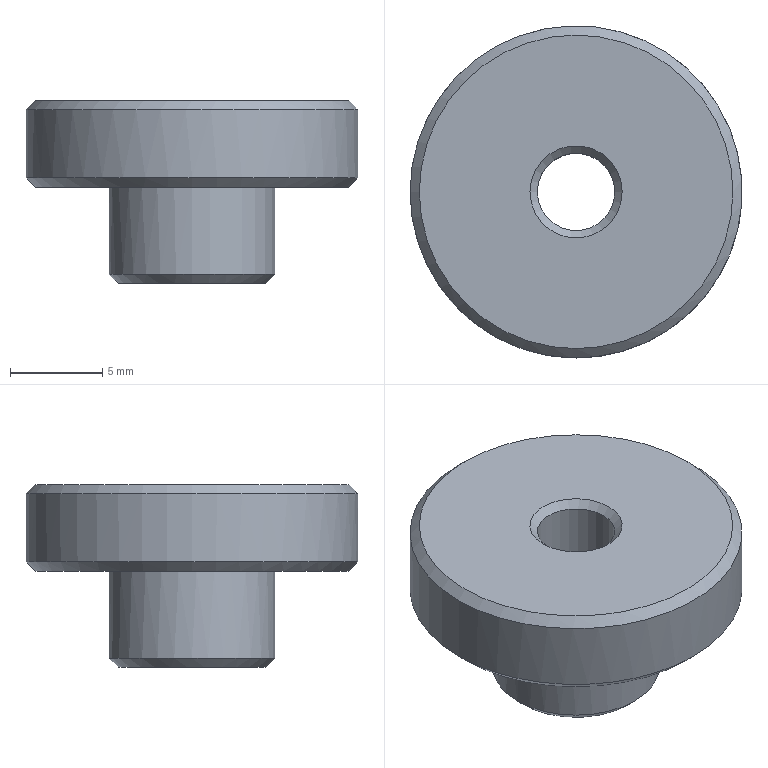Part | STEP file | 1 solid | 11 faces | box 18 x 18 x 9.92 mm | volume 1371 mm3 | cone 5 | cylinder 3 | plane 3 | commonest cylinder face diameters 4.2 x1 9 x1 18 x1
STEP:
#1=CARTESIAN_POINT('',(0.,0.,0.));
#2=DIRECTION('',(0.,0.,1.));
#3=DIRECTION('',(1.,0.,0.));
#4=AXIS2_PLACEMENT_3D('',#1,#2,#3);
#5=CARTESIAN_POINT('',(1716.457,442.48,-42.801));
#6=VERTEX_POINT('',#5);
#7=CARTESIAN_POINT('',(1720.957,437.98,-42.801));
#8=VERTEX_POINT('',#7);
#9=CARTESIAN_POINT('',(1720.957,442.48,-42.801));
#10=DIRECTION('',(0.,0.,1.));
#11=DIRECTION('',(-1.,0.,0.));
#12=AXIS2_PLACEMENT_3D('',#9,#10,#11);
#13=CIRCLE('',#12,4.5);
#14=CARTESIAN_POINT('',(1720.957,442.48,-44.081));
#15=DIRECTION('',(0.,0.,1.));
#16=DIRECTION('',(1.,0.,0.));
#17=AXIS2_PLACEMENT_3D('',#14,#15,#16);
#18=CYLINDRICAL_SURFACE('',#17,4.5);
#19=CARTESIAN_POINT('',(9.425,1.28));
#20=DIRECTION('',(1.,0.));
#21=VECTOR('',#20,1.);
#22=LINE('',#19,#21);
#23=(GEOMETRIC_REPRESENTATION_CONTEXT(2)PARAMETRIC_REPRESENTATION_CONTEXT()REPRESENTATION_CONTEXT('',''));
#24=DEFINITIONAL_REPRESENTATION('',(#22),#23);
#25=PCURVE('',#18,#24);
#26=CARTESIAN_POINT('',(1720.957,442.48,-43.301));
#27=DIRECTION('',(0.,0.,1.));
#28=DIRECTION('',(1.,0.,0.));
#29=AXIS2_PLACEMENT_3D('',#26,#27,#28);
#30=CONICAL_SURFACE('',#29,4.,0.7854);
#31=CARTESIAN_POINT('',(9.425,0.5));
#32=DIRECTION('',(1.,0.));
#33=VECTOR('',#32,1.);
#34=LINE('',#31,#33);
#35=(GEOMETRIC_REPRESENTATION_CONTEXT(2)PARAMETRIC_REPRESENTATION_CONTEXT()REPRESENTATION_CONTEXT('',''));
#36=DEFINITIONAL_REPRESENTATION('',(#34),#35);
#37=PCURVE('',#30,#36);
#38=SURFACE_CURVE('',#13,(#25,#37),.PCURVE_S1.);
#39=EDGE_CURVE('',#6,#8,#38,.T.);
#40=ORIENTED_EDGE('',*,*,#39,.T.);
#41=CARTESIAN_POINT('',(1720.957,437.98,-38.081));
#42=VERTEX_POINT('',#41);
#43=CARTESIAN_POINT('',(1720.957,437.98,-42.801));
#44=CARTESIAN_POINT('',(1720.957,437.98,-38.081));
#45=B_SPLINE_CURVE_WITH_KNOTS('',1,(#43,#44),.UNSPECIFIED.,.F.,.F.,(2,2),(1.28,6.),.PIECEWISE_BEZIER_KNOTS.);
#46=CARTESIAN_POINT('',(10.996,0.));
#47=DIRECTION('',(0.,1.));
#48=VECTOR('',#47,1.);
#49=LINE('',#46,#48);
#50=(GEOMETRIC_REPRESENTATION_CONTEXT(2)PARAMETRIC_REPRESENTATION_CONTEXT()REPRESENTATION_CONTEXT('',''));
#51=DEFINITIONAL_REPRESENTATION('',(#49),#50);
#52=PCURVE('',#18,#51);
#53=CARTESIAN_POINT('',(4.712,0.));
#54=DIRECTION('',(0.,1.));
#55=VECTOR('',#54,1.);
#56=LINE('',#53,#55);
#57=(GEOMETRIC_REPRESENTATION_CONTEXT(2)PARAMETRIC_REPRESENTATION_CONTEXT()REPRESENTATION_CONTEXT('',''));
#58=DEFINITIONAL_REPRESENTATION('',(#56),#57);
#59=PCURVE('',#18,#58);
#60=SEAM_CURVE('',#45,(#52,#59),.PCURVE_S1.);
#61=EDGE_CURVE('',#8,#42,#60,.T.);
#62=ORIENTED_EDGE('',*,*,#61,.T.);
#63=CARTESIAN_POINT('',(1720.957,442.48,-38.081));
#64=DIRECTION('',(0.,0.,-1.));
#65=DIRECTION('',(0.,-1.,0.));
#66=AXIS2_PLACEMENT_3D('',#63,#64,#65);
#67=CIRCLE('',#66,4.5);
#68=CARTESIAN_POINT('',(10.996,6.));
#69=DIRECTION('',(-1.,0.));
#70=VECTOR('',#69,1.);
#71=LINE('',#68,#70);
#72=(GEOMETRIC_REPRESENTATION_CONTEXT(2)PARAMETRIC_REPRESENTATION_CONTEXT()REPRESENTATION_CONTEXT('',''));
#73=DEFINITIONAL_REPRESENTATION('',(#71),#72);
#74=PCURVE('',#18,#73);
#75=CARTESIAN_POINT('',(1720.957,442.48,-38.081));
#76=DIRECTION('',(0.,0.,-1.));
#77=DIRECTION('',(0.,-1.,0.));
#78=AXIS2_PLACEMENT_3D('',#75,#76,#77);
#79=PLANE('',#78);
#80=CARTESIAN_POINT('',(0.,0.));
#81=DIRECTION('',(1.,0.));
#82=AXIS2_PLACEMENT_2D('',#80,#81);
#83=CIRCLE('',#82,4.5);
#84=(GEOMETRIC_REPRESENTATION_CONTEXT(2)PARAMETRIC_REPRESENTATION_CONTEXT()REPRESENTATION_CONTEXT('',''));
#85=DEFINITIONAL_REPRESENTATION('',(#83),#84);
#86=PCURVE('',#79,#85);
#87=SURFACE_CURVE('',#67,(#74,#86),.PCURVE_S1.);
#88=EDGE_CURVE('',#42,#42,#87,.T.);
#89=ORIENTED_EDGE('',*,*,#88,.T.);
#90=ORIENTED_EDGE('',*,*,#61,.F.);
#91=CARTESIAN_POINT('',(1720.957,442.48,-42.801));
#92=DIRECTION('',(0.,0.,1.));
#93=DIRECTION('',(-1.,0.,0.));
#94=AXIS2_PLACEMENT_3D('',#91,#92,#93);
#95=CIRCLE('',#94,4.5);
#96=CARTESIAN_POINT('',(3.142,1.28));
#97=DIRECTION('',(1.,0.));
#98=VECTOR('',#97,1.);
#99=LINE('',#96,#98);
#100=(GEOMETRIC_REPRESENTATION_CONTEXT(2)PARAMETRIC_REPRESENTATION_CONTEXT()REPRESENTATION_CONTEXT('',''));
#101=DEFINITIONAL_REPRESENTATION('',(#99),#100);
#102=PCURVE('',#18,#101);
#103=CARTESIAN_POINT('',(3.142,0.5));
#104=DIRECTION('',(1.,0.));
#105=VECTOR('',#104,1.);
#106=LINE('',#103,#105);
#107=(GEOMETRIC_REPRESENTATION_CONTEXT(2)PARAMETRIC_REPRESENTATION_CONTEXT()REPRESENTATION_CONTEXT('',''));
#108=DEFINITIONAL_REPRESENTATION('',(#106),#107);
#109=PCURVE('',#30,#108);
#110=SURFACE_CURVE('',#95,(#102,#109),.PCURVE_S1.);
#111=EDGE_CURVE('',#8,#6,#110,.T.);
#112=ORIENTED_EDGE('',*,*,#111,.T.);
#113=EDGE_LOOP('',(#40,#62,#89,#90,#112));
#114=FACE_BOUND('',#113,.T.);
#115=ADVANCED_FACE('',(#114),#18,.T.);
#116=CARTESIAN_POINT('',(1720.957,439.98,-43.301));
#117=VERTEX_POINT('',#116);
#118=CARTESIAN_POINT('',(1718.457,442.48,-43.301));
#119=VERTEX_POINT('',#118);
#120=CARTESIAN_POINT('',(1720.957,442.48,-43.301));
#121=DIRECTION('',(0.,0.,1.));
#122=DIRECTION('',(0.,-1.,0.));
#123=AXIS2_PLACEMENT_3D('',#120,#121,#122);
#124=CIRCLE('',#123,2.5);
#125=CARTESIAN_POINT('',(1720.957,442.48,-43.301));
#126=DIRECTION('',(0.,0.,-1.));
#127=DIRECTION('',(0.,-1.,0.));
#128=AXIS2_PLACEMENT_3D('',#125,#126,#127);
#129=PLANE('',#128);
#130=CARTESIAN_POINT('',(2.5,0.));
#131=CARTESIAN_POINT('',(2.5,-4.33));
#132=CARTESIAN_POINT('',(-1.25,-2.165));
#133=CARTESIAN_POINT('',(-5.,0.));
#134=CARTESIAN_POINT('',(-1.25,2.165));
#135=CARTESIAN_POINT('',(2.5,4.33));
#136=CARTESIAN_POINT('',(2.5,0.));
#137=(BOUNDED_CURVE()B_SPLINE_CURVE(2,(#130,#131,#132,#133,#134,#135,#136),.UNSPECIFIED.,.T.,.F.)B_SPLINE_CURVE_WITH_KNOTS((1,2,2,2,2,1),(-2.094,0.,2.094,4.189,6.283,8.378),.UNSPECIFIED.)CURVE()GEOMETRIC_REPRESENTATION_ITEM()RATIONAL_B_SPLINE_CURVE((1.,0.5,1.,0.5,1.,0.5,1.))REPRESENTATION_ITEM(''));
#138=(GEOMETRIC_REPRESENTATION_CONTEXT(2)PARAMETRIC_REPRESENTATION_CONTEXT()REPRESENTATION_CONTEXT('',''));
#139=DEFINITIONAL_REPRESENTATION('',(#137),#138);
#140=PCURVE('',#129,#139);
#141=CARTESIAN_POINT('',(1720.957,442.48,-43.301));
#142=DIRECTION('',(0.,0.,-1.));
#143=DIRECTION('',(-1.,0.,0.));
#144=AXIS2_PLACEMENT_3D('',#141,#142,#143);
#145=CONICAL_SURFACE('',#144,2.5,0.7854);
#146=CARTESIAN_POINT('',(4.712,0.));
#147=DIRECTION('',(-1.,0.));
#148=VECTOR('',#147,1.);
#149=LINE('',#146,#148);
#150=(GEOMETRIC_REPRESENTATION_CONTEXT(2)PARAMETRIC_REPRESENTATION_CONTEXT()REPRESENTATION_CONTEXT('',''));
#151=DEFINITIONAL_REPRESENTATION('',(#149),#150);
#152=PCURVE('',#145,#151);
#153=SURFACE_CURVE('',#124,(#140,#152),.PCURVE_S1.);
#154=EDGE_CURVE('',#117,#119,#153,.T.);
#155=ORIENTED_EDGE('',*,*,#154,.T.);
#156=CARTESIAN_POINT('',(1720.957,442.48,-43.301));
#157=DIRECTION('',(0.,0.,1.));
#158=DIRECTION('',(0.,-1.,0.));
#159=AXIS2_PLACEMENT_3D('',#156,#157,#158);
#160=CIRCLE('',#159,2.5);
#161=CARTESIAN_POINT('',(2.5,0.));
#162=CARTESIAN_POINT('',(2.5,-4.33));
#163=CARTESIAN_POINT('',(-1.25,-2.165));
#164=CARTESIAN_POINT('',(-5.,0.));
#165=CARTESIAN_POINT('',(-1.25,2.165));
#166=CARTESIAN_POINT('',(2.5,4.33));
#167=CARTESIAN_POINT('',(2.5,0.));
#168=(BOUNDED_CURVE()B_SPLINE_CURVE(2,(#161,#162,#163,#164,#165,#166,#167),.UNSPECIFIED.,.T.,.F.)B_SPLINE_CURVE_WITH_KNOTS((1,2,2,2,2,1),(-2.094,0.,2.094,4.189,6.283,8.378),.UNSPECIFIED.)CURVE()GEOMETRIC_REPRESENTATION_ITEM()RATIONAL_B_SPLINE_CURVE((1.,0.5,1.,0.5,1.,0.5,1.))REPRESENTATION_ITEM(''));
#169=(GEOMETRIC_REPRESENTATION_CONTEXT(2)PARAMETRIC_REPRESENTATION_CONTEXT()REPRESENTATION_CONTEXT('',''));
#170=DEFINITIONAL_REPRESENTATION('',(#168),#169);
#171=PCURVE('',#129,#170);
#172=CARTESIAN_POINT('',(10.996,0.));
#173=DIRECTION('',(-1.,0.));
#174=VECTOR('',#173,1.);
#175=LINE('',#172,#174);
#176=(GEOMETRIC_REPRESENTATION_CONTEXT(2)PARAMETRIC_REPRESENTATION_CONTEXT()REPRESENTATION_CONTEXT('',''));
#177=DEFINITIONAL_REPRESENTATION('',(#175),#176);
#178=PCURVE('',#145,#177);
#179=SURFACE_CURVE('',#160,(#171,#178),.PCURVE_S1.);
#180=EDGE_CURVE('',#119,#117,#179,.T.);
#181=ORIENTED_EDGE('',*,*,#180,.T.);
#182=EDGE_LOOP('',(#155,#181));
#183=FACE_BOUND('',#182,.T.);
#184=CARTESIAN_POINT('',(1720.957,438.48,-43.301));
#185=VERTEX_POINT('',#184);
#186=CARTESIAN_POINT('',(1720.957,442.48,-43.301));
#187=DIRECTION('',(0.,0.,-1.));
#188=DIRECTION('',(0.,-1.,0.));
#189=AXIS2_PLACEMENT_3D('',#186,#187,#188);
#190=CIRCLE('',#189,4.);
#191=CARTESIAN_POINT('',(0.,0.));
#192=DIRECTION('',(1.,0.));
#193=AXIS2_PLACEMENT_2D('',#191,#192);
#194=CIRCLE('',#193,4.);
#195=(GEOMETRIC_REPRESENTATION_CONTEXT(2)PARAMETRIC_REPRESENTATION_CONTEXT()REPRESENTATION_CONTEXT('',''));
#196=DEFINITIONAL_REPRESENTATION('',(#194),#195);
#197=PCURVE('',#129,#196);
#198=CARTESIAN_POINT('',(10.996,0.));
#199=DIRECTION('',(-1.,0.));
#200=VECTOR('',#199,1.);
#201=LINE('',#198,#200);
#202=(GEOMETRIC_REPRESENTATION_CONTEXT(2)PARAMETRIC_REPRESENTATION_CONTEXT()REPRESENTATION_CONTEXT('',''));
#203=DEFINITIONAL_REPRESENTATION('',(#201),#202);
#204=PCURVE('',#30,#203);
#205=SURFACE_CURVE('',#190,(#197,#204),.PCURVE_S1.);
#206=EDGE_CURVE('',#185,#185,#205,.T.);
#207=ORIENTED_EDGE('',*,*,#206,.T.);
#208=EDGE_LOOP('',(#207));
#209=FACE_BOUND('',#208,.T.);
#210=ADVANCED_FACE('',(#183,#209),#129,.T.);
#211=CARTESIAN_POINT('',(1711.957,442.48,-33.881));
#212=VERTEX_POINT('',#211);
#213=CARTESIAN_POINT('',(1720.957,442.48,-33.881));
#214=DIRECTION('',(0.,0.,-1.));
#215=DIRECTION('',(-1.,0.,0.));
#216=AXIS2_PLACEMENT_3D('',#213,#214,#215);
#217=CIRCLE('',#216,9.);
#218=CARTESIAN_POINT('',(1720.957,442.48,-37.881));
#219=DIRECTION('',(0.,0.,1.));
#220=DIRECTION('',(1.,0.,0.));
#221=AXIS2_PLACEMENT_3D('',#218,#219,#220);
#222=CYLINDRICAL_SURFACE('',#221,9.);
#223=CARTESIAN_POINT('',(9.425,4.));
#224=DIRECTION('',(-1.,0.));
#225=VECTOR('',#224,1.);
#226=LINE('',#223,#225);
#227=(GEOMETRIC_REPRESENTATION_CONTEXT(2)PARAMETRIC_REPRESENTATION_CONTEXT()REPRESENTATION_CONTEXT('',''));
#228=DEFINITIONAL_REPRESENTATION('',(#226),#227);
#229=PCURVE('',#222,#228);
#230=CARTESIAN_POINT('',(1720.957,442.48,-33.881));
#231=DIRECTION('',(0.,0.,-1.));
#232=DIRECTION('',(-1.,0.,0.));
#233=AXIS2_PLACEMENT_3D('',#230,#231,#232);
#234=CONICAL_SURFACE('',#233,9.,0.7854);
#235=CARTESIAN_POINT('',(0.,0.));
#236=DIRECTION('',(1.,0.));
#237=VECTOR('',#236,1.);
#238=LINE('',#235,#237);
#239=(GEOMETRIC_REPRESENTATION_CONTEXT(2)PARAMETRIC_REPRESENTATION_CONTEXT()REPRESENTATION_CONTEXT('',''));
#240=DEFINITIONAL_REPRESENTATION('',(#238),#239);
#241=PCURVE('',#234,#240);
#242=SURFACE_CURVE('',#217,(#229,#241),.PCURVE_S1.);
#243=EDGE_CURVE('',#212,#212,#242,.T.);
#244=ORIENTED_EDGE('',*,*,#243,.T.);
#245=CARTESIAN_POINT('',(1711.957,442.48,-37.581));
#246=VERTEX_POINT('',#245);
#247=CARTESIAN_POINT('',(1711.957,442.48,-37.581));
#248=CARTESIAN_POINT('',(1711.957,442.48,-33.881));
#249=B_SPLINE_CURVE_WITH_KNOTS('',1,(#247,#248),.UNSPECIFIED.,.F.,.F.,(2,2),(0.3,4.),.PIECEWISE_BEZIER_KNOTS.);
#250=CARTESIAN_POINT('',(3.142,0.));
#251=DIRECTION('',(0.,1.));
#252=VECTOR('',#251,1.);
#253=LINE('',#250,#252);
#254=(GEOMETRIC_REPRESENTATION_CONTEXT(2)PARAMETRIC_REPRESENTATION_CONTEXT()REPRESENTATION_CONTEXT('',''));
#255=DEFINITIONAL_REPRESENTATION('',(#253),#254);
#256=PCURVE('',#222,#255);
#257=CARTESIAN_POINT('',(9.425,0.));
#258=DIRECTION('',(0.,1.));
#259=VECTOR('',#258,1.);
#260=LINE('',#257,#259);
#261=(GEOMETRIC_REPRESENTATION_CONTEXT(2)PARAMETRIC_REPRESENTATION_CONTEXT()REPRESENTATION_CONTEXT('',''));
#262=DEFINITIONAL_REPRESENTATION('',(#260),#261);
#263=PCURVE('',#222,#262);
#264=SEAM_CURVE('',#249,(#256,#263),.PCURVE_S1.);
#265=EDGE_CURVE('',#246,#212,#264,.T.);
#266=ORIENTED_EDGE('',*,*,#265,.F.);
#267=CARTESIAN_POINT('',(1720.957,433.48,-37.581));
#268=VERTEX_POINT('',#267);
#269=CARTESIAN_POINT('',(1720.957,442.48,-37.581));
#270=DIRECTION('',(0.,0.,1.));
#271=DIRECTION('',(-1.,0.,0.));
#272=AXIS2_PLACEMENT_3D('',#269,#270,#271);
#273=CIRCLE('',#272,9.);
#274=CARTESIAN_POINT('',(3.142,0.3));
#275=DIRECTION('',(1.,0.));
#276=VECTOR('',#275,1.);
#277=LINE('',#274,#276);
#278=(GEOMETRIC_REPRESENTATION_CONTEXT(2)PARAMETRIC_REPRESENTATION_CONTEXT()REPRESENTATION_CONTEXT('',''));
#279=DEFINITIONAL_REPRESENTATION('',(#277),#278);
#280=PCURVE('',#222,#279);
#281=CARTESIAN_POINT('',(1720.957,442.48,-38.081));
#282=DIRECTION('',(0.,0.,1.));
#283=DIRECTION('',(1.,0.,0.));
#284=AXIS2_PLACEMENT_3D('',#281,#282,#283);
#285=CONICAL_SURFACE('',#284,8.5,0.7854);
#286=CARTESIAN_POINT('',(9.425,0.5));
#287=DIRECTION('',(1.,0.));
#288=VECTOR('',#287,1.);
#289=LINE('',#286,#288);
#290=(GEOMETRIC_REPRESENTATION_CONTEXT(2)PARAMETRIC_REPRESENTATION_CONTEXT()REPRESENTATION_CONTEXT('',''));
#291=DEFINITIONAL_REPRESENTATION('',(#289),#290);
#292=PCURVE('',#285,#291);
#293=SURFACE_CURVE('',#273,(#280,#292),.PCURVE_S1.);
#294=EDGE_CURVE('',#246,#268,#293,.T.);
#295=ORIENTED_EDGE('',*,*,#294,.T.);
#296=CARTESIAN_POINT('',(1720.957,442.48,-37.581));
#297=DIRECTION('',(0.,0.,1.));
#298=DIRECTION('',(-1.,0.,0.));
#299=AXIS2_PLACEMENT_3D('',#296,#297,#298);
#300=CIRCLE('',#299,9.);
#301=CARTESIAN_POINT('',(3.142,0.3));
#302=DIRECTION('',(1.,0.));
#303=VECTOR('',#302,1.);
#304=LINE('',#301,#303);
#305=(GEOMETRIC_REPRESENTATION_CONTEXT(2)PARAMETRIC_REPRESENTATION_CONTEXT()REPRESENTATION_CONTEXT('',''));
#306=DEFINITIONAL_REPRESENTATION('',(#304),#305);
#307=PCURVE('',#222,#306);
#308=CARTESIAN_POINT('',(3.142,0.5));
#309=DIRECTION('',(1.,0.));
#310=VECTOR('',#309,1.);
#311=LINE('',#308,#310);
#312=(GEOMETRIC_REPRESENTATION_CONTEXT(2)PARAMETRIC_REPRESENTATION_CONTEXT()REPRESENTATION_CONTEXT('',''));
#313=DEFINITIONAL_REPRESENTATION('',(#311),#312);
#314=PCURVE('',#285,#313);
#315=SURFACE_CURVE('',#300,(#307,#314),.PCURVE_S1.);
#316=EDGE_CURVE('',#268,#246,#315,.T.);
#317=ORIENTED_EDGE('',*,*,#316,.T.);
#318=ORIENTED_EDGE('',*,*,#265,.T.);
#319=EDGE_LOOP('',(#244,#266,#295,#317,#318));
#320=FACE_BOUND('',#319,.T.);
#321=ADVANCED_FACE('',(#320),#222,.T.);
#322=CARTESIAN_POINT('',(1720.957,433.98,-38.081));
#323=VERTEX_POINT('',#322);
#324=CARTESIAN_POINT('',(1720.957,442.48,-38.081));
#325=DIRECTION('',(0.,0.,-1.));
#326=DIRECTION('',(0.,-1.,0.));
#327=AXIS2_PLACEMENT_3D('',#324,#325,#326);
#328=CIRCLE('',#327,8.5);
#329=CARTESIAN_POINT('',(0.,0.));
#330=DIRECTION('',(1.,0.));
#331=AXIS2_PLACEMENT_2D('',#329,#330);
#332=CIRCLE('',#331,8.5);
#333=(GEOMETRIC_REPRESENTATION_CONTEXT(2)PARAMETRIC_REPRESENTATION_CONTEXT()REPRESENTATION_CONTEXT('',''));
#334=DEFINITIONAL_REPRESENTATION('',(#332),#333);
#335=PCURVE('',#79,#334);
#336=CARTESIAN_POINT('',(10.996,0.));
#337=DIRECTION('',(-1.,0.));
#338=VECTOR('',#337,1.);
#339=LINE('',#336,#338);
#340=(GEOMETRIC_REPRESENTATION_CONTEXT(2)PARAMETRIC_REPRESENTATION_CONTEXT()REPRESENTATION_CONTEXT('',''));
#341=DEFINITIONAL_REPRESENTATION('',(#339),#340);
#342=PCURVE('',#285,#341);
#343=SURFACE_CURVE('',#328,(#335,#342),.PCURVE_S1.);
#344=EDGE_CURVE('',#323,#323,#343,.T.);
#345=ORIENTED_EDGE('',*,*,#344,.T.);
#346=EDGE_LOOP('',(#345));
#347=FACE_BOUND('',#346,.T.);
#348=ORIENTED_EDGE('',*,*,#88,.F.);
#349=EDGE_LOOP('',(#348));
#350=FACE_BOUND('',#349,.T.);
#351=ADVANCED_FACE('',(#347,#350),#79,.T.);
#352=CARTESIAN_POINT('',(1723.457,442.48,-33.381));
#353=VERTEX_POINT('',#352);
#354=CARTESIAN_POINT('',(1720.957,442.48,-33.381));
#355=DIRECTION('',(0.,0.,-1.));
#356=DIRECTION('',(1.,0.,0.));
#357=AXIS2_PLACEMENT_3D('',#354,#355,#356);
#358=CIRCLE('',#357,2.5);
#359=CARTESIAN_POINT('',(1706.957,452.48,-33.381));
#360=DIRECTION('',(0.,0.,1.));
#361=DIRECTION('',(1.,0.,0.));
#362=AXIS2_PLACEMENT_3D('',#359,#360,#361);
#363=PLANE('',#362);
#364=CARTESIAN_POINT('',(16.5,-10.));
#365=CARTESIAN_POINT('',(16.5,-14.33));
#366=CARTESIAN_POINT('',(12.75,-12.165));
#367=CARTESIAN_POINT('',(9.,-10.));
#368=CARTESIAN_POINT('',(12.75,-7.835));
#369=CARTESIAN_POINT('',(16.5,-5.67));
#370=CARTESIAN_POINT('',(16.5,-10.));
#371=(BOUNDED_CURVE()B_SPLINE_CURVE(2,(#364,#365,#366,#367,#368,#369,#370),.UNSPECIFIED.,.T.,.F.)B_SPLINE_CURVE_WITH_KNOTS((1,2,2,2,2,1),(-2.094,0.,2.094,4.189,6.283,8.378),.UNSPECIFIED.)CURVE()GEOMETRIC_REPRESENTATION_ITEM()RATIONAL_B_SPLINE_CURVE((1.,0.5,1.,0.5,1.,0.5,1.))REPRESENTATION_ITEM(''));
#372=(GEOMETRIC_REPRESENTATION_CONTEXT(2)PARAMETRIC_REPRESENTATION_CONTEXT()REPRESENTATION_CONTEXT('',''));
#373=DEFINITIONAL_REPRESENTATION('',(#371),#372);
#374=PCURVE('',#363,#373);
#375=CARTESIAN_POINT('',(1720.957,442.48,-33.381));
#376=DIRECTION('',(0.,0.,1.));
#377=DIRECTION('',(1.,0.,0.));
#378=AXIS2_PLACEMENT_3D('',#375,#376,#377);
#379=CONICAL_SURFACE('',#378,2.5,0.7854);
#380=CARTESIAN_POINT('',(6.283,0.));
#381=DIRECTION('',(-1.,0.));
#382=VECTOR('',#381,1.);
#383=LINE('',#380,#382);
#384=(GEOMETRIC_REPRESENTATION_CONTEXT(2)PARAMETRIC_REPRESENTATION_CONTEXT()REPRESENTATION_CONTEXT('',''));
#385=DEFINITIONAL_REPRESENTATION('',(#383),#384);
#386=PCURVE('',#379,#385);
#387=SURFACE_CURVE('',#358,(#374,#386),.PCURVE_S1.);
#388=EDGE_CURVE('',#353,#353,#387,.T.);
#389=ORIENTED_EDGE('',*,*,#388,.T.);
#390=EDGE_LOOP('',(#389));
#391=FACE_BOUND('',#390,.T.);
#392=CARTESIAN_POINT('',(1729.457,442.48,-33.381));
#393=VERTEX_POINT('',#392);
#394=CARTESIAN_POINT('',(1712.457,442.48,-33.381));
#395=VERTEX_POINT('',#394);
#396=CARTESIAN_POINT('',(1720.957,442.48,-33.381));
#397=DIRECTION('',(0.,0.,1.));
#398=DIRECTION('',(1.,0.,0.));
#399=AXIS2_PLACEMENT_3D('',#396,#397,#398);
#400=CIRCLE('',#399,8.5);
#401=CARTESIAN_POINT('',(14.,-10.));
#402=DIRECTION('',(1.,0.));
#403=AXIS2_PLACEMENT_2D('',#401,#402);
#404=CIRCLE('',#403,8.5);
#405=(GEOMETRIC_REPRESENTATION_CONTEXT(2)PARAMETRIC_REPRESENTATION_CONTEXT()REPRESENTATION_CONTEXT('',''));
#406=DEFINITIONAL_REPRESENTATION('',(#404),#405);
#407=PCURVE('',#363,#406);
#408=CARTESIAN_POINT('',(3.142,-0.5));
#409=DIRECTION('',(-1.,0.));
#410=VECTOR('',#409,1.);
#411=LINE('',#408,#410);
#412=(GEOMETRIC_REPRESENTATION_CONTEXT(2)PARAMETRIC_REPRESENTATION_CONTEXT()REPRESENTATION_CONTEXT('',''));
#413=DEFINITIONAL_REPRESENTATION('',(#411),#412);
#414=PCURVE('',#234,#413);
#415=SURFACE_CURVE('',#400,(#407,#414),.PCURVE_S1.);
#416=EDGE_CURVE('',#393,#395,#415,.T.);
#417=ORIENTED_EDGE('',*,*,#416,.T.);
#418=CARTESIAN_POINT('',(1720.957,442.48,-33.381));
#419=DIRECTION('',(0.,0.,1.));
#420=DIRECTION('',(1.,0.,0.));
#421=AXIS2_PLACEMENT_3D('',#418,#419,#420);
#422=CIRCLE('',#421,8.5);
#423=CARTESIAN_POINT('',(14.,-10.));
#424=DIRECTION('',(1.,0.));
#425=AXIS2_PLACEMENT_2D('',#423,#424);
#426=CIRCLE('',#425,8.5);
#427=(GEOMETRIC_REPRESENTATION_CONTEXT(2)PARAMETRIC_REPRESENTATION_CONTEXT()REPRESENTATION_CONTEXT('',''));
#428=DEFINITIONAL_REPRESENTATION('',(#426),#427);
#429=PCURVE('',#363,#428);
#430=CARTESIAN_POINT('',(9.425,-0.5));
#431=DIRECTION('',(-1.,0.));
#432=VECTOR('',#431,1.);
#433=LINE('',#430,#432);
#434=(GEOMETRIC_REPRESENTATION_CONTEXT(2)PARAMETRIC_REPRESENTATION_CONTEXT()REPRESENTATION_CONTEXT('',''));
#435=DEFINITIONAL_REPRESENTATION('',(#433),#434);
#436=PCURVE('',#234,#435);
#437=SURFACE_CURVE('',#422,(#429,#436),.PCURVE_S1.);
#438=EDGE_CURVE('',#395,#393,#437,.T.);
#439=ORIENTED_EDGE('',*,*,#438,.T.);
#440=EDGE_LOOP('',(#417,#439));
#441=FACE_BOUND('',#440,.T.);
#442=ADVANCED_FACE('',(#391,#441),#363,.T.);
#443=ORIENTED_EDGE('',*,*,#39,.F.);
#444=ORIENTED_EDGE('',*,*,#111,.F.);
#445=CARTESIAN_POINT('',(1720.957,438.48,-43.301));
#446=CARTESIAN_POINT('',(1720.957,437.98,-42.801));
#447=B_SPLINE_CURVE_WITH_KNOTS('',1,(#445,#446),.UNSPECIFIED.,.F.,.F.,(2,2),(0.,0.7071),.PIECEWISE_BEZIER_KNOTS.);
#448=CARTESIAN_POINT('',(4.712,0.));
#449=DIRECTION('',(0.,1.));
#450=VECTOR('',#449,1.);
#451=LINE('',#448,#450);
#452=(GEOMETRIC_REPRESENTATION_CONTEXT(2)PARAMETRIC_REPRESENTATION_CONTEXT()REPRESENTATION_CONTEXT('',''));
#453=DEFINITIONAL_REPRESENTATION('',(#451),#452);
#454=PCURVE('',#30,#453);
#455=CARTESIAN_POINT('',(10.996,0.));
#456=DIRECTION('',(0.,1.));
#457=VECTOR('',#456,1.);
#458=LINE('',#455,#457);
#459=(GEOMETRIC_REPRESENTATION_CONTEXT(2)PARAMETRIC_REPRESENTATION_CONTEXT()REPRESENTATION_CONTEXT('',''));
#460=DEFINITIONAL_REPRESENTATION('',(#458),#459);
#461=PCURVE('',#30,#460);
#462=SEAM_CURVE('',#447,(#454,#461),.PCURVE_S1.);
#463=EDGE_CURVE('',#185,#8,#462,.T.);
#464=ORIENTED_EDGE('',*,*,#463,.F.);
#465=ORIENTED_EDGE('',*,*,#206,.F.);
#466=ORIENTED_EDGE('',*,*,#463,.T.);
#467=EDGE_LOOP('',(#443,#444,#464,#465,#466));
#468=FACE_BOUND('',#467,.T.);
#469=ADVANCED_FACE('',(#468),#30,.T.);
#470=ORIENTED_EDGE('',*,*,#438,.F.);
#471=CARTESIAN_POINT('',(1712.457,442.48,-33.381));
#472=CARTESIAN_POINT('',(1711.957,442.48,-33.881));
#473=B_SPLINE_CURVE_WITH_KNOTS('',1,(#471,#472),.UNSPECIFIED.,.F.,.F.,(2,2),(-0.7071,0.),.PIECEWISE_BEZIER_KNOTS.);
#474=CARTESIAN_POINT('',(6.283,0.));
#475=DIRECTION('',(0.,1.));
#476=VECTOR('',#475,1.);
#477=LINE('',#474,#476);
#478=(GEOMETRIC_REPRESENTATION_CONTEXT(2)PARAMETRIC_REPRESENTATION_CONTEXT()REPRESENTATION_CONTEXT('',''));
#479=DEFINITIONAL_REPRESENTATION('',(#477),#478);
#480=PCURVE('',#234,#479);
#481=CARTESIAN_POINT('',(0.,0.));
#482=DIRECTION('',(0.,1.));
#483=VECTOR('',#482,1.);
#484=LINE('',#481,#483);
#485=(GEOMETRIC_REPRESENTATION_CONTEXT(2)PARAMETRIC_REPRESENTATION_CONTEXT()REPRESENTATION_CONTEXT('',''));
#486=DEFINITIONAL_REPRESENTATION('',(#484),#485);
#487=PCURVE('',#234,#486);
#488=SEAM_CURVE('',#473,(#480,#487),.PCURVE_S1.);
#489=EDGE_CURVE('',#395,#212,#488,.T.);
#490=ORIENTED_EDGE('',*,*,#489,.T.);
#491=ORIENTED_EDGE('',*,*,#243,.F.);
#492=ORIENTED_EDGE('',*,*,#489,.F.);
#493=ORIENTED_EDGE('',*,*,#416,.F.);
#494=EDGE_LOOP('',(#470,#490,#491,#492,#493));
#495=FACE_BOUND('',#494,.T.);
#496=ADVANCED_FACE('',(#495),#234,.T.);
#497=ORIENTED_EDGE('',*,*,#316,.F.);
#498=CARTESIAN_POINT('',(1720.957,433.98,-38.081));
#499=CARTESIAN_POINT('',(1720.957,433.48,-37.581));
#500=B_SPLINE_CURVE_WITH_KNOTS('',1,(#498,#499),.UNSPECIFIED.,.F.,.F.,(2,2),(0.,0.7071),.PIECEWISE_BEZIER_KNOTS.);
#501=CARTESIAN_POINT('',(4.712,0.));
#502=DIRECTION('',(0.,1.));
#503=VECTOR('',#502,1.);
#504=LINE('',#501,#503);
#505=(GEOMETRIC_REPRESENTATION_CONTEXT(2)PARAMETRIC_REPRESENTATION_CONTEXT()REPRESENTATION_CONTEXT('',''));
#506=DEFINITIONAL_REPRESENTATION('',(#504),#505);
#507=PCURVE('',#285,#506);
#508=CARTESIAN_POINT('',(10.996,0.));
#509=DIRECTION('',(0.,1.));
#510=VECTOR('',#509,1.);
#511=LINE('',#508,#510);
#512=(GEOMETRIC_REPRESENTATION_CONTEXT(2)PARAMETRIC_REPRESENTATION_CONTEXT()REPRESENTATION_CONTEXT('',''));
#513=DEFINITIONAL_REPRESENTATION('',(#511),#512);
#514=PCURVE('',#285,#513);
#515=SEAM_CURVE('',#500,(#507,#514),.PCURVE_S1.);
#516=EDGE_CURVE('',#323,#268,#515,.T.);
#517=ORIENTED_EDGE('',*,*,#516,.F.);
#518=ORIENTED_EDGE('',*,*,#344,.F.);
#519=ORIENTED_EDGE('',*,*,#516,.T.);
#520=ORIENTED_EDGE('',*,*,#294,.F.);
#521=EDGE_LOOP('',(#497,#517,#518,#519,#520));
#522=FACE_BOUND('',#521,.T.);
#523=ADVANCED_FACE('',(#522),#285,.T.);
#524=CARTESIAN_POINT('',(1718.857,442.48,-33.781));
#525=VERTEX_POINT('',#524);
#526=CARTESIAN_POINT('',(1723.057,442.48,-33.781));
#527=VERTEX_POINT('',#526);
#528=CARTESIAN_POINT('',(1720.957,442.48,-33.781));
#529=DIRECTION('',(0.,0.,1.));
#530=DIRECTION('',(-1.,0.,0.));
#531=AXIS2_PLACEMENT_3D('',#528,#529,#530);
#532=CIRCLE('',#531,2.1);
#533=CARTESIAN_POINT('',(1720.957,442.48,-43.301));
#534=DIRECTION('',(0.,0.,1.));
#535=DIRECTION('',(0.,1.,0.));
#536=AXIS2_PLACEMENT_3D('',#533,#534,#535);
#537=CYLINDRICAL_SURFACE('',#536,2.1);
#538=CARTESIAN_POINT('',(1.571,9.52));
#539=DIRECTION('',(1.,0.));
#540=VECTOR('',#539,1.);
#541=LINE('',#538,#540);
#542=(GEOMETRIC_REPRESENTATION_CONTEXT(2)PARAMETRIC_REPRESENTATION_CONTEXT()REPRESENTATION_CONTEXT('',''));
#543=DEFINITIONAL_REPRESENTATION('',(#541),#542);
#544=PCURVE('',#537,#543);
#545=CARTESIAN_POINT('',(3.142,-0.4));
#546=DIRECTION('',(1.,0.));
#547=VECTOR('',#546,1.);
#548=LINE('',#545,#547);
#549=(GEOMETRIC_REPRESENTATION_CONTEXT(2)PARAMETRIC_REPRESENTATION_CONTEXT()REPRESENTATION_CONTEXT('',''));
#550=DEFINITIONAL_REPRESENTATION('',(#548),#549);
#551=PCURVE('',#379,#550);
#552=SURFACE_CURVE('',#532,(#544,#551),.PCURVE_S1.);
#553=EDGE_CURVE('',#525,#527,#552,.T.);
#554=ORIENTED_EDGE('',*,*,#553,.F.);
#555=CARTESIAN_POINT('',(1718.857,442.48,-42.901));
#556=VERTEX_POINT('',#555);
#557=CARTESIAN_POINT('',(1718.857,442.48,-42.901));
#558=CARTESIAN_POINT('',(1718.857,442.48,-33.781));
#559=B_SPLINE_CURVE_WITH_KNOTS('',1,(#557,#558),.UNSPECIFIED.,.F.,.F.,(2,2),(0.4,9.52),.PIECEWISE_BEZIER_KNOTS.);
#560=CARTESIAN_POINT('',(1.571,0.));
#561=DIRECTION('',(0.,1.));
#562=VECTOR('',#561,1.);
#563=LINE('',#560,#562);
#564=(GEOMETRIC_REPRESENTATION_CONTEXT(2)PARAMETRIC_REPRESENTATION_CONTEXT()REPRESENTATION_CONTEXT('',''));
#565=DEFINITIONAL_REPRESENTATION('',(#563),#564);
#566=PCURVE('',#537,#565);
#567=CARTESIAN_POINT('',(7.854,0.));
#568=DIRECTION('',(0.,1.));
#569=VECTOR('',#568,1.);
#570=LINE('',#567,#569);
#571=(GEOMETRIC_REPRESENTATION_CONTEXT(2)PARAMETRIC_REPRESENTATION_CONTEXT()REPRESENTATION_CONTEXT('',''));
#572=DEFINITIONAL_REPRESENTATION('',(#570),#571);
#573=PCURVE('',#537,#572);
#574=SEAM_CURVE('',#559,(#566,#573),.PCURVE_S1.);
#575=EDGE_CURVE('',#556,#525,#574,.T.);
#576=ORIENTED_EDGE('',*,*,#575,.F.);
#577=CARTESIAN_POINT('',(1720.957,442.48,-42.901));
#578=DIRECTION('',(0.,0.,-1.));
#579=DIRECTION('',(-1.,0.,0.));
#580=AXIS2_PLACEMENT_3D('',#577,#578,#579);
#581=CIRCLE('',#580,2.1);
#582=CARTESIAN_POINT('',(7.854,0.4));
#583=DIRECTION('',(-1.,0.));
#584=VECTOR('',#583,1.);
#585=LINE('',#582,#584);
#586=(GEOMETRIC_REPRESENTATION_CONTEXT(2)PARAMETRIC_REPRESENTATION_CONTEXT()REPRESENTATION_CONTEXT('',''));
#587=DEFINITIONAL_REPRESENTATION('',(#585),#586);
#588=PCURVE('',#537,#587);
#589=CARTESIAN_POINT('',(0.,-0.4));
#590=DIRECTION('',(1.,0.));
#591=VECTOR('',#590,1.);
#592=LINE('',#589,#591);
#593=(GEOMETRIC_REPRESENTATION_CONTEXT(2)PARAMETRIC_REPRESENTATION_CONTEXT()REPRESENTATION_CONTEXT('',''));
#594=DEFINITIONAL_REPRESENTATION('',(#592),#593);
#595=PCURVE('',#145,#594);
#596=SURFACE_CURVE('',#581,(#588,#595),.PCURVE_S1.);
#597=EDGE_CURVE('',#556,#556,#596,.T.);
#598=ORIENTED_EDGE('',*,*,#597,.F.);
#599=ORIENTED_EDGE('',*,*,#575,.T.);
#600=CARTESIAN_POINT('',(1720.957,442.48,-33.781));
#601=DIRECTION('',(0.,0.,1.));
#602=DIRECTION('',(-1.,0.,0.));
#603=AXIS2_PLACEMENT_3D('',#600,#601,#602);
#604=CIRCLE('',#603,2.1);
#605=CARTESIAN_POINT('',(1.571,9.52));
#606=DIRECTION('',(1.,0.));
#607=VECTOR('',#606,1.);
#608=LINE('',#605,#607);
#609=(GEOMETRIC_REPRESENTATION_CONTEXT(2)PARAMETRIC_REPRESENTATION_CONTEXT()REPRESENTATION_CONTEXT('',''));
#610=DEFINITIONAL_REPRESENTATION('',(#608),#609);
#611=PCURVE('',#537,#610);
#612=CARTESIAN_POINT('',(-3.142,-0.4));
#613=DIRECTION('',(1.,0.));
#614=VECTOR('',#613,1.);
#615=LINE('',#612,#614);
#616=(GEOMETRIC_REPRESENTATION_CONTEXT(2)PARAMETRIC_REPRESENTATION_CONTEXT()REPRESENTATION_CONTEXT('',''));
#617=DEFINITIONAL_REPRESENTATION('',(#615),#616);
#618=PCURVE('',#379,#617);
#619=SURFACE_CURVE('',#604,(#611,#618),.PCURVE_S1.);
#620=EDGE_CURVE('',#527,#525,#619,.T.);
#621=ORIENTED_EDGE('',*,*,#620,.F.);
#622=EDGE_LOOP('',(#554,#576,#598,#599,#621));
#623=FACE_BOUND('',#622,.F.);
#624=ADVANCED_FACE('',(#623),#537,.F.);
#625=ORIENTED_EDGE('',*,*,#597,.T.);
#626=CARTESIAN_POINT('',(1718.857,442.48,-42.901));
#627=CARTESIAN_POINT('',(1718.457,442.48,-43.301));
#628=B_SPLINE_CURVE_WITH_KNOTS('',1,(#626,#627),.UNSPECIFIED.,.F.,.F.,(2,2),(-0.5657,0.),.PIECEWISE_BEZIER_KNOTS.);
#629=CARTESIAN_POINT('',(6.283,0.));
#630=DIRECTION('',(0.,1.));
#631=VECTOR('',#630,1.);
#632=LINE('',#629,#631);
#633=(GEOMETRIC_REPRESENTATION_CONTEXT(2)PARAMETRIC_REPRESENTATION_CONTEXT()REPRESENTATION_CONTEXT('',''));
#634=DEFINITIONAL_REPRESENTATION('',(#632),#633);
#635=PCURVE('',#145,#634);
#636=CARTESIAN_POINT('',(0.,0.));
#637=DIRECTION('',(0.,1.));
#638=VECTOR('',#637,1.);
#639=LINE('',#636,#638);
#640=(GEOMETRIC_REPRESENTATION_CONTEXT(2)PARAMETRIC_REPRESENTATION_CONTEXT()REPRESENTATION_CONTEXT('',''));
#641=DEFINITIONAL_REPRESENTATION('',(#639),#640);
#642=PCURVE('',#145,#641);
#643=SEAM_CURVE('',#628,(#635,#642),.PCURVE_S1.);
#644=EDGE_CURVE('',#556,#119,#643,.T.);
#645=ORIENTED_EDGE('',*,*,#644,.T.);
#646=ORIENTED_EDGE('',*,*,#180,.T.);
#647=ORIENTED_EDGE('',*,*,#154,.T.);
#648=ORIENTED_EDGE('',*,*,#644,.F.);
#649=EDGE_LOOP('',(#625,#645,#646,#647,#648));
#650=FACE_BOUND('',#649,.F.);
#651=ADVANCED_FACE('',(#650),#145,.F.);
#652=ORIENTED_EDGE('',*,*,#553,.T.);
#653=CARTESIAN_POINT('',(1723.057,442.48,-33.781));
#654=CARTESIAN_POINT('',(1723.457,442.48,-33.381));
#655=B_SPLINE_CURVE_WITH_KNOTS('',1,(#653,#654),.UNSPECIFIED.,.F.,.F.,(2,2),(-0.5657,0.),.PIECEWISE_BEZIER_KNOTS.);
#656=CARTESIAN_POINT('',(6.283,0.));
#657=DIRECTION('',(0.,1.));
#658=VECTOR('',#657,1.);
#659=LINE('',#656,#658);
#660=(GEOMETRIC_REPRESENTATION_CONTEXT(2)PARAMETRIC_REPRESENTATION_CONTEXT()REPRESENTATION_CONTEXT('',''));
#661=DEFINITIONAL_REPRESENTATION('',(#659),#660);
#662=PCURVE('',#379,#661);
#663=CARTESIAN_POINT('',(0.,0.));
#664=DIRECTION('',(0.,1.));
#665=VECTOR('',#664,1.);
#666=LINE('',#663,#665);
#667=(GEOMETRIC_REPRESENTATION_CONTEXT(2)PARAMETRIC_REPRESENTATION_CONTEXT()REPRESENTATION_CONTEXT('',''));
#668=DEFINITIONAL_REPRESENTATION('',(#666),#667);
#669=PCURVE('',#379,#668);
#670=SEAM_CURVE('',#655,(#662,#669),.PCURVE_S1.);
#671=EDGE_CURVE('',#527,#353,#670,.T.);
#672=ORIENTED_EDGE('',*,*,#671,.T.);
#673=ORIENTED_EDGE('',*,*,#388,.T.);
#674=ORIENTED_EDGE('',*,*,#671,.F.);
#675=ORIENTED_EDGE('',*,*,#620,.T.);
#676=EDGE_LOOP('',(#652,#672,#673,#674,#675));
#677=FACE_BOUND('',#676,.F.);
#678=ADVANCED_FACE('',(#677),#379,.F.);
#679=CLOSED_SHELL('',(#115,#210,#321,#351,#442,#469,#496,#523,#624,#651,#678));
#680=MANIFOLD_SOLID_BREP('',#679);
#681=(LENGTH_UNIT()NAMED_UNIT(*)SI_UNIT(.MILLI.,.METRE.));
#682=UNCERTAINTY_MEASURE_WITH_UNIT(LENGTH_MEASURE(0.000005),#681,'','');
#683=(NAMED_UNIT(*)PLANE_ANGLE_UNIT()SI_UNIT($,.RADIAN.));
#684=(NAMED_UNIT(*)SI_UNIT($,.STERADIAN.)SOLID_ANGLE_UNIT());
#685=(GEOMETRIC_REPRESENTATION_CONTEXT(3)GLOBAL_UNCERTAINTY_ASSIGNED_CONTEXT((#682))GLOBAL_UNIT_ASSIGNED_CONTEXT((#681,#683,#684))REPRESENTATION_CONTEXT('',''));
#686=ADVANCED_BREP_SHAPE_REPRESENTATION('',(#4,#680),#685);